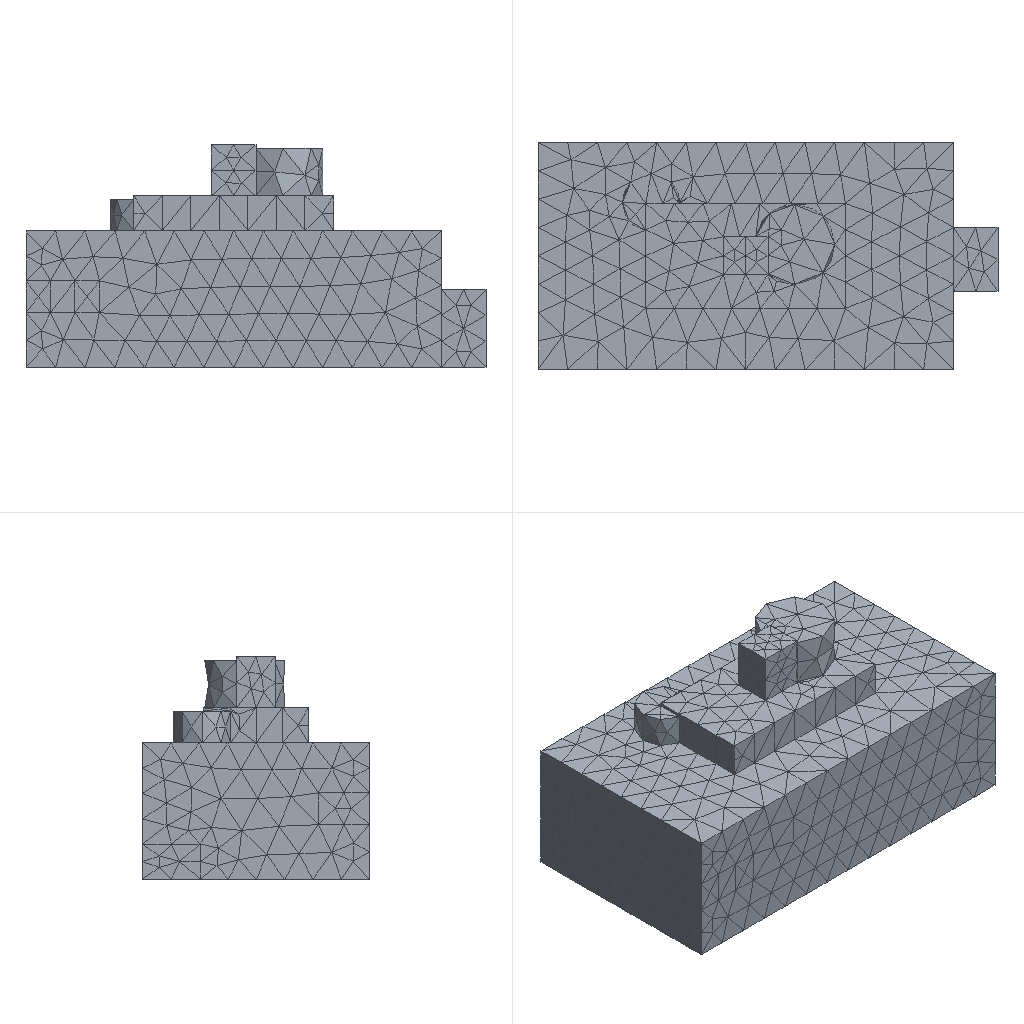Simulation study | ansys mapdl
Set-up summary:
category,name,step,type,value,unit,region
solver,ansys_mapdl
units,mm-N-s-tonne (MPa),,inferred,E=210000 density=
analysis,model,,static
mesh,nodes,,,8709
mesh,elements,,,5490
element_type,SOLID187,,,5490
material,mat 1,,E,210000
material,mat 1,,nu,0.3
load,,model,body load temp,,,all
load,,model,force,"1000 [dir=(0, 0, -1) n=508]",,node list
bc,,model,fixed,"[dofs=UX,UY,UZ n=8912]",,node list
Ansys APDL input file, long lists of numbers shortened:
/COM,ANSYS RELEASE 2026 R1           BUILD 26.1      UP20260202       09:09:58
/PREP7
/NOPR
/TITLE,2
ANTYPE, 0
*IF,_CDRDOFF,EQ,1,THEN     !if solid model was read in
_CDRDOFF=             !reset flag, numoffs already performed
*ELSE              !offset database for the following FE model
NUMOFF,NODE,     8709
NUMOFF,ELEM,     5490
NUMOFF,MAT ,        1
NUMOFF,TYPE,        1
*ENDIF
*SET,_RETURN ,  0.
*SET,_STATUS ,  0.
*SET,_UIQR   ,  508.
*SET,__FLOATPARAMETER__,  8709.
DOF,DELETE
ETBLOCK,        1,        1
(2i9,19a9)
        1      187        0        0        0        0        0        0        0        0        0        0        0        0        0        0        0        0        0        0        0
       -1
NBLOCK,6,SOLID,      8709,      8709
(3i9,6e21.13e3)
        1        0        0 7.0000000000000E+000 6.0000000000000E+000 6.9710000000000E+001
! (8708 more lines like these left out)
N,UNBL,LOC,       -1,
EBLOCK,19,SOLID,      5490,      5490
(19i10)
         1         1         1         1         0         0         0         0        10         0         1      2683      2684      2685      2686      3286      3287      3288      3289
! (10979 more lines like these left out)
        -1
MPTEMP,UNBL, 1, 1,  0.    ,
MPDATA,UNBL, 1,EX  ,       1, 1,  210000.000    ,
MPTEMP,UNBL, 1, 1,  0.    ,
MPDATA,UNBL, 1,NUXY,       1, 1, 0.3    ,
MPTEMP,UNBL, 1, 1,  0.    ,
MPDATA,UNBL, 1,PRXY,       1, 1, 0.3    ,
EXTOPT,ATTR,      0,      0,      0
EXTOPT,ESIZE,  0,  0.
EXTOPT,ACLEAR,      0
TREF,  0.
IRLF,  0
BFUNIF,TEMP,_TINY
ACEL,  0.    ,  0.    ,  0.
OMEGA,  0.    ,  0.    ,  0.
DOMEGA,  0.    ,  0.    ,  0.
CGLOC,  0.    ,  0.    ,  0.
CGOMEGA,  0.    ,  0.    ,  0.
DCGOMG,  0.    ,  0.    ,  0.
KUSE,     0
TIME,  0.
ALPHAD,  0.
BETAD,  0.
DMPRAT,  0.
DMPSTR,  0.
CRPLIM, 0.1    ,   0
CRPLIM,  0.    ,   1
NCNV,     0, 1.000000000E+12,     0,  0.    ,  0.
NEQIT,     0
ERESX,DEFA
DBLOCK,      8912
(i9,a6,2(pg16.9))
      536  UX    0.00000000      0.00000000
! (8911 more lines like these left out)
       -1
FBLOCK,       508
(i9,a6,2(pg16.9))
        1  FZ   -1.96850394      0.00000000
! (507 more lines like these left out)
       -1
/GO
FINISH
Results summary:
result,analysis_type_db,,,static,unstated
result,n_sets,,,1,unstated
result,load_steps[0].set,load_step=1,,1,unstated
result,load_steps[0].substep,load_step=1,,1,unstated
result,load_steps[0].time,load_step=1,,1,unstated
result,load_steps[0].freq,load_step=1,,1,unstated
result,load_steps[0].max_usum,load_step=1,,0.0003218,unstated
result,load_steps[0].max_seqv,load_step=1,,3.676,unstated
result,load_steps[0].reaction_sum.FX,load_step=1,,-1.42881e-11,unstated
result,load_steps[0].reaction_sum.FY,load_step=1,,-2.50804e-11,unstated
result,load_steps[0].reaction_sum.FZ,load_step=1,,1000,unstated
result,load_steps[0].reaction_sum.MX,load_step=1,,0,unstated
result,load_steps[0].reaction_sum.MY,load_step=1,,0,unstated
result,load_steps[0].reaction_sum.MZ,load_step=1,,0,unstated
result,convergence,,,results present for all listed sets,unstated